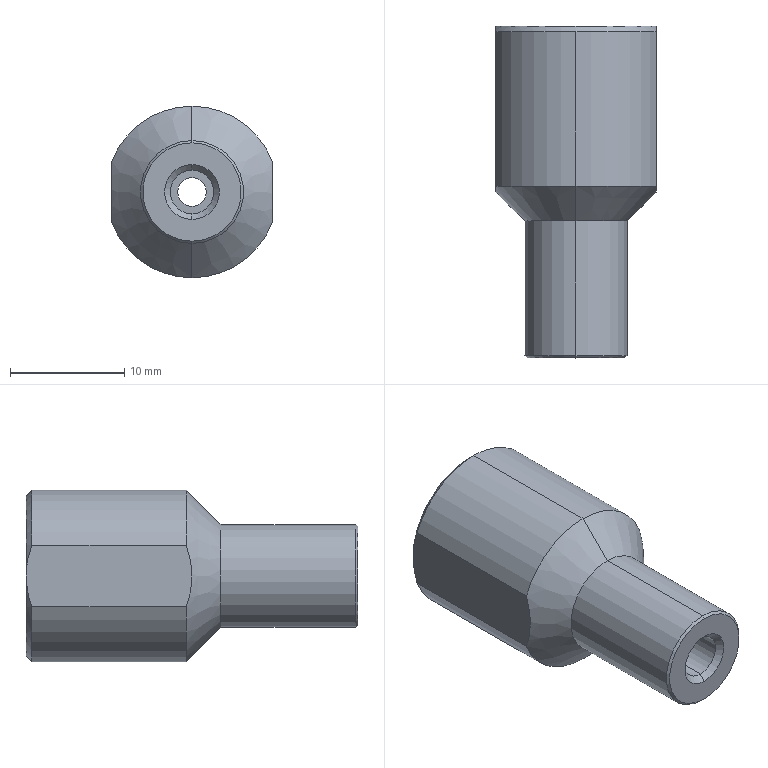Part | SolidWorks | features Chamfer 4, ICE 4, Extrusion 1, HoleWzd 1 | 1 solid | 27 faces | box 14 x 29 x 15 mm | volume 2672 mm3 | cylinder 11 | cone 11 | plane 5 | commonest cylinder face diameters 15 x3 2.5 x2 3.8 x2 8.5 x2 9 x2
STEP:
#1=CARTESIAN_POINT('',(0.,-12.,-4.25));
#2=VERTEX_POINT('',#1);
#3=CARTESIAN_POINT('',(0.,-12.,4.25));
#4=VERTEX_POINT('',#3);
#5=CARTESIAN_POINT('',(0.,-12.,0.));
#6=DIRECTION('',(0.,1.,0.));
#7=DIRECTION('',(0.,0.,1.));
#8=AXIS2_PLACEMENT_3D('',#5,#6,#7);
#9=CIRCLE('',#8,4.25);
#10=EDGE_CURVE('',#2,#4,#9,.T.);
#11=ORIENTED_EDGE('',*,*,#10,.F.);
#12=CARTESIAN_POINT('',(0.,0.,-4.25));
#13=VERTEX_POINT('',#12);
#14=CARTESIAN_POINT('',(0.,0.,-4.25));
#15=DIRECTION('',(0.,1.,0.));
#16=VECTOR('',#15,1000.);
#17=LINE('',#14,#16);
#18=EDGE_CURVE('',#2,#13,#17,.T.);
#19=ORIENTED_EDGE('',*,*,#18,.T.);
#20=CARTESIAN_POINT('',(0.,0.,4.25));
#21=VERTEX_POINT('',#20);
#22=CARTESIAN_POINT('',(0.,0.,0.));
#23=DIRECTION('',(0.,1.,0.));
#24=DIRECTION('',(0.,0.,1.));
#25=AXIS2_PLACEMENT_3D('',#22,#23,#24);
#26=CIRCLE('',#25,4.25);
#27=EDGE_CURVE('',#13,#21,#26,.T.);
#28=ORIENTED_EDGE('',*,*,#27,.T.);
#29=CARTESIAN_POINT('',(0.,0.,4.25));
#30=DIRECTION('',(0.,1.,0.));
#31=VECTOR('',#30,1000.);
#32=LINE('',#29,#31);
#33=EDGE_CURVE('',#4,#21,#32,.T.);
#34=ORIENTED_EDGE('',*,*,#33,.F.);
#35=EDGE_LOOP('',(#11,#19,#28,#34));
#36=FACE_OUTER_BOUND('',#35,.T.);
#37=CARTESIAN_POINT('',(0.,0.,0.));
#38=DIRECTION('',(0.,1.,0.));
#39=DIRECTION('',(0.,0.,1.));
#40=AXIS2_PLACEMENT_3D('',#37,#38,#39);
#41=CYLINDRICAL_SURFACE('',#40,4.25);
#42=ADVANCED_FACE('',(#36),#41,.F.);
#43=CARTESIAN_POINT('',(0.,-13.803,-1.25));
#44=VERTEX_POINT('',#43);
#45=CARTESIAN_POINT('',(0.,-13.803,1.25));
#46=VERTEX_POINT('',#45);
#47=CARTESIAN_POINT('',(0.,-13.803,0.));
#48=DIRECTION('',(0.,1.,0.));
#49=DIRECTION('',(0.,0.,1.));
#50=AXIS2_PLACEMENT_3D('',#47,#48,#49);
#51=CIRCLE('',#50,1.25);
#52=EDGE_CURVE('',#44,#46,#51,.T.);
#53=ORIENTED_EDGE('',*,*,#52,.F.);
#54=CARTESIAN_POINT('',(0.,-12.,-4.25));
#55=DIRECTION('',(0.,0.515,-0.8572));
#56=VECTOR('',#55,1000.);
#57=LINE('',#54,#56);
#58=EDGE_CURVE('',#44,#2,#57,.T.);
#59=ORIENTED_EDGE('',*,*,#58,.T.);
#60=ORIENTED_EDGE('',*,*,#10,.T.);
#61=CARTESIAN_POINT('',(0.,-12.,4.25));
#62=DIRECTION('',(0.,0.515,0.8572));
#63=VECTOR('',#62,1000.);
#64=LINE('',#61,#63);
#65=EDGE_CURVE('',#46,#4,#64,.T.);
#66=ORIENTED_EDGE('',*,*,#65,.F.);
#67=EDGE_LOOP('',(#53,#59,#60,#66));
#68=FACE_OUTER_BOUND('',#67,.T.);
#69=CARTESIAN_POINT('',(0.,-12.,0.));
#70=DIRECTION('',(0.,1.,0.));
#71=DIRECTION('',(0.,0.,1.));
#72=AXIS2_PLACEMENT_3D('',#69,#70,#71);
#73=CONICAL_SURFACE('',#72,4.25,1.03);
#74=ADVANCED_FACE('',(#68),#73,.F.);
#75=CARTESIAN_POINT('',(0.,-29.,-4.3));
#76=VERTEX_POINT('',#75);
#77=CARTESIAN_POINT('',(0.,-29.,4.3));
#78=VERTEX_POINT('',#77);
#79=CARTESIAN_POINT('',(0.,-29.,0.));
#80=DIRECTION('',(0.,-1.,0.));
#81=DIRECTION('',(0.,0.,-1.));
#82=AXIS2_PLACEMENT_3D('',#79,#80,#81);
#83=CIRCLE('',#82,4.3);
#84=EDGE_CURVE('',#76,#78,#83,.T.);
#85=ORIENTED_EDGE('',*,*,#84,.F.);
#86=CARTESIAN_POINT('',(0.,-28.8,-4.5));
#87=VERTEX_POINT('',#86);
#88=CARTESIAN_POINT('',(0.,-29.,-4.3));
#89=DIRECTION('',(0.,0.7071,-0.7071));
#90=VECTOR('',#89,1000.);
#91=LINE('',#88,#90);
#92=EDGE_CURVE('',#76,#87,#91,.T.);
#93=ORIENTED_EDGE('',*,*,#92,.T.);
#94=CARTESIAN_POINT('',(0.,-28.8,4.5));
#95=VERTEX_POINT('',#94);
#96=CARTESIAN_POINT('',(0.,-28.8,0.));
#97=DIRECTION('',(0.,1.,0.));
#98=DIRECTION('',(0.,0.,-1.));
#99=AXIS2_PLACEMENT_3D('',#96,#97,#98);
#100=CIRCLE('',#99,4.5);
#101=EDGE_CURVE('',#95,#87,#100,.T.);
#102=ORIENTED_EDGE('',*,*,#101,.F.);
#103=CARTESIAN_POINT('',(0.,-29.,4.3));
#104=DIRECTION('',(0.,0.7071,0.7071));
#105=VECTOR('',#104,1000.);
#106=LINE('',#103,#105);
#107=EDGE_CURVE('',#78,#95,#106,.T.);
#108=ORIENTED_EDGE('',*,*,#107,.F.);
#109=EDGE_LOOP('',(#85,#93,#102,#108));
#110=FACE_OUTER_BOUND('',#109,.T.);
#111=CARTESIAN_POINT('',(0.,-29.,0.));
#112=DIRECTION('',(0.,1.,0.));
#113=DIRECTION('',(0.,0.,1.));
#114=AXIS2_PLACEMENT_3D('',#111,#112,#113);
#115=CONICAL_SURFACE('',#114,4.3,0.7854);
#116=ADVANCED_FACE('',(#110),#115,.T.);
#117=CARTESIAN_POINT('',(0.,-28.5,1.9));
#118=VERTEX_POINT('',#117);
#119=CARTESIAN_POINT('',(0.,-28.5,-1.9));
#120=VERTEX_POINT('',#119);
#121=CARTESIAN_POINT('',(0.,-28.5,0.));
#122=DIRECTION('',(0.,-1.,0.));
#123=DIRECTION('',(0.,0.,-1.));
#124=AXIS2_PLACEMENT_3D('',#121,#122,#123);
#125=CIRCLE('',#124,1.9);
#126=EDGE_CURVE('',#118,#120,#125,.T.);
#127=ORIENTED_EDGE('',*,*,#126,.F.);
#128=CARTESIAN_POINT('',(0.,-29.,2.4));
#129=VERTEX_POINT('',#128);
#130=CARTESIAN_POINT('',(0.,-28.5,1.9));
#131=DIRECTION('',(0.,-0.7071,0.7071));
#132=VECTOR('',#131,1000.);
#133=LINE('',#130,#132);
#134=EDGE_CURVE('',#118,#129,#133,.T.);
#135=ORIENTED_EDGE('',*,*,#134,.T.);
#136=CARTESIAN_POINT('',(0.,-29.,-2.4));
#137=VERTEX_POINT('',#136);
#138=CARTESIAN_POINT('',(0.,-29.,0.));
#139=DIRECTION('',(0.,1.,0.));
#140=DIRECTION('',(0.,0.,-1.));
#141=AXIS2_PLACEMENT_3D('',#138,#139,#140);
#142=CIRCLE('',#141,2.4);
#143=EDGE_CURVE('',#137,#129,#142,.T.);
#144=ORIENTED_EDGE('',*,*,#143,.F.);
#145=CARTESIAN_POINT('',(0.,-28.5,-1.9));
#146=DIRECTION('',(0.,-0.7071,-0.7071));
#147=VECTOR('',#146,1000.);
#148=LINE('',#145,#147);
#149=EDGE_CURVE('',#120,#137,#148,.T.);
#150=ORIENTED_EDGE('',*,*,#149,.F.);
#151=EDGE_LOOP('',(#127,#135,#144,#150));
#152=FACE_OUTER_BOUND('',#151,.T.);
#153=CARTESIAN_POINT('',(0.,-28.5,0.));
#154=DIRECTION('',(0.,-1.,0.));
#155=DIRECTION('',(0.,0.,-1.));
#156=AXIS2_PLACEMENT_3D('',#153,#154,#155);
#157=CONICAL_SURFACE('',#156,1.9,0.7854);
#158=ADVANCED_FACE('',(#152),#157,.F.);
#159=ORIENTED_EDGE('',*,*,#52,.T.);
#160=CARTESIAN_POINT('',(0.,-21.,1.25));
#161=VERTEX_POINT('',#160);
#162=CARTESIAN_POINT('',(0.,0.,1.25));
#163=DIRECTION('',(0.,-1.,0.));
#164=VECTOR('',#163,1000.);
#165=LINE('',#162,#164);
#166=EDGE_CURVE('',#46,#161,#165,.T.);
#167=ORIENTED_EDGE('',*,*,#166,.T.);
#168=CARTESIAN_POINT('',(0.,-21.,-1.25));
#169=VERTEX_POINT('',#168);
#170=CARTESIAN_POINT('',(0.,-21.,0.));
#171=DIRECTION('',(0.,-1.,0.));
#172=DIRECTION('',(0.,0.,-1.));
#173=AXIS2_PLACEMENT_3D('',#170,#171,#172);
#174=CIRCLE('',#173,1.25);
#175=EDGE_CURVE('',#161,#169,#174,.T.);
#176=ORIENTED_EDGE('',*,*,#175,.T.);
#177=CARTESIAN_POINT('',(0.,0.,-1.25));
#178=DIRECTION('',(0.,-1.,0.));
#179=VECTOR('',#178,1000.);
#180=LINE('',#177,#179);
#181=EDGE_CURVE('',#44,#169,#180,.T.);
#182=ORIENTED_EDGE('',*,*,#181,.F.);
#183=EDGE_LOOP('',(#159,#167,#176,#182));
#184=FACE_OUTER_BOUND('',#183,.T.);
#185=CARTESIAN_POINT('',(0.,0.,0.));
#186=DIRECTION('',(0.,-1.,0.));
#187=DIRECTION('',(0.,0.,-1.));
#188=AXIS2_PLACEMENT_3D('',#185,#186,#187);
#189=CYLINDRICAL_SURFACE('',#188,1.25);
#190=ADVANCED_FACE('',(#184),#189,.F.);
#191=CARTESIAN_POINT('',(0.,-17.,-4.5));
#192=VERTEX_POINT('',#191);
#193=CARTESIAN_POINT('',(0.,-17.,4.5));
#194=VERTEX_POINT('',#193);
#195=CARTESIAN_POINT('',(0.,-17.,0.));
#196=DIRECTION('',(0.,-1.,0.));
#197=DIRECTION('',(0.,0.,1.));
#198=AXIS2_PLACEMENT_3D('',#195,#196,#197);
#199=CIRCLE('',#198,4.5);
#200=EDGE_CURVE('',#192,#194,#199,.T.);
#201=ORIENTED_EDGE('',*,*,#200,.F.);
#202=CARTESIAN_POINT('',(0.,-14.,-7.5));
#203=VERTEX_POINT('',#202);
#204=CARTESIAN_POINT('',(0.,-14.,-7.5));
#205=DIRECTION('',(0.,0.7071,-0.7071));
#206=VECTOR('',#205,1000.);
#207=LINE('',#204,#206);
#208=EDGE_CURVE('',#192,#203,#207,.T.);
#209=ORIENTED_EDGE('',*,*,#208,.T.);
#210=CARTESIAN_POINT('',(7.,-14.,-2.693));
#211=VERTEX_POINT('',#210);
#212=CARTESIAN_POINT('',(0.,-14.,0.));
#213=DIRECTION('',(0.,1.,0.));
#214=DIRECTION('',(0.,0.,1.));
#215=AXIS2_PLACEMENT_3D('',#212,#213,#214);
#216=CIRCLE('',#215,7.5);
#217=EDGE_CURVE('',#211,#203,#216,.T.);
#218=ORIENTED_EDGE('',*,*,#217,.F.);
#219=CARTESIAN_POINT('',(7.,-14.,2.693));
#220=VERTEX_POINT('',#219);
#221=CARTESIAN_POINT('',(7.,-14.,2.693));
#222=CARTESIAN_POINT('',(7.,-14.155,2.26));
#223=CARTESIAN_POINT('',(7.,-14.282,1.816));
#224=CARTESIAN_POINT('',(7.,-14.453,0.9207));
#225=CARTESIAN_POINT('',(7.,-14.5,0.4668));
#226=CARTESIAN_POINT('',(7.,-14.5,-0.2249));
#227=CARTESIAN_POINT('',(7.,-14.489,-0.4564));
#228=CARTESIAN_POINT('',(7.,-14.444,-0.9134));
#229=CARTESIAN_POINT('',(7.,-14.411,-1.14));
#230=CARTESIAN_POINT('',(7.,-14.325,-1.59));
#231=CARTESIAN_POINT('',(7.,-14.272,-1.813));
#232=CARTESIAN_POINT('',(7.,-14.148,-2.257));
#233=CARTESIAN_POINT('',(7.,-14.077,-2.477));
#234=CARTESIAN_POINT('',(7.,-14.,-2.693));
#235=B_SPLINE_CURVE_WITH_KNOTS('',3,(#221,#222,#223,#224,#225,#226,#227,#228,#229,#230,#231,#232,#233,#234),.UNSPECIFIED.,.F.,.F.,(4,2,2,2,2,2,4),(0.02883,0.03019,0.03156,0.03224,0.03292,0.0336,0.03428),.UNSPECIFIED.);
#236=EDGE_CURVE('',#220,#211,#235,.T.);
#237=ORIENTED_EDGE('',*,*,#236,.F.);
#238=CARTESIAN_POINT('',(0.,-14.,7.5));
#239=VERTEX_POINT('',#238);
#240=CARTESIAN_POINT('',(0.,-14.,0.));
#241=DIRECTION('',(0.,1.,0.));
#242=DIRECTION('',(0.,0.,1.));
#243=AXIS2_PLACEMENT_3D('',#240,#241,#242);
#244=CIRCLE('',#243,7.5);
#245=EDGE_CURVE('',#239,#220,#244,.T.);
#246=ORIENTED_EDGE('',*,*,#245,.F.);
#247=CARTESIAN_POINT('',(0.,-14.,7.5));
#248=DIRECTION('',(0.,0.7071,0.7071));
#249=VECTOR('',#248,1000.);
#250=LINE('',#247,#249);
#251=EDGE_CURVE('',#194,#239,#250,.T.);
#252=ORIENTED_EDGE('',*,*,#251,.F.);
#253=EDGE_LOOP('',(#201,#209,#218,#237,#246,#252));
#254=FACE_OUTER_BOUND('',#253,.T.);
#255=CARTESIAN_POINT('',(0.,-14.,0.));
#256=DIRECTION('',(0.,1.,0.));
#257=DIRECTION('',(0.,0.,1.));
#258=AXIS2_PLACEMENT_3D('',#255,#256,#257);
#259=CONICAL_SURFACE('',#258,7.5,0.7854);
#260=ADVANCED_FACE('',(#254),#259,.T.);
#261=CARTESIAN_POINT('',(0.,-21.,1.9));
#262=VERTEX_POINT('',#261);
#263=CARTESIAN_POINT('',(0.,-21.,-1.9));
#264=VERTEX_POINT('',#263);
#265=CARTESIAN_POINT('',(0.,-21.,0.));
#266=DIRECTION('',(0.,-1.,0.));
#267=DIRECTION('',(0.,0.,-1.));
#268=AXIS2_PLACEMENT_3D('',#265,#266,#267);
#269=CIRCLE('',#268,1.9);
#270=EDGE_CURVE('',#262,#264,#269,.T.);
#271=ORIENTED_EDGE('',*,*,#270,.F.);
#272=CARTESIAN_POINT('',(0.,-21.,1.9));
#273=DIRECTION('',(0.,-1.,0.));
#274=VECTOR('',#273,1000.);
#275=LINE('',#272,#274);
#276=EDGE_CURVE('',#262,#118,#275,.T.);
#277=ORIENTED_EDGE('',*,*,#276,.T.);
#278=ORIENTED_EDGE('',*,*,#126,.T.);
#279=CARTESIAN_POINT('',(0.,-21.,-1.9));
#280=DIRECTION('',(0.,-1.,0.));
#281=VECTOR('',#280,1000.);
#282=LINE('',#279,#281);
#283=EDGE_CURVE('',#264,#120,#282,.T.);
#284=ORIENTED_EDGE('',*,*,#283,.F.);
#285=EDGE_LOOP('',(#271,#277,#278,#284));
#286=FACE_OUTER_BOUND('',#285,.T.);
#287=CARTESIAN_POINT('',(0.,-21.,0.));
#288=DIRECTION('',(0.,-1.,0.));
#289=DIRECTION('',(0.,0.,-1.));
#290=AXIS2_PLACEMENT_3D('',#287,#288,#289);
#291=CYLINDRICAL_SURFACE('',#290,1.9);
#292=ADVANCED_FACE('',(#286),#291,.F.);
#293=ORIENTED_EDGE('',*,*,#101,.T.);
#294=CARTESIAN_POINT('',(0.,-29.,-4.5));
#295=DIRECTION('',(0.,1.,0.));
#296=VECTOR('',#295,1000.);
#297=LINE('',#294,#296);
#298=EDGE_CURVE('',#87,#192,#297,.T.);
#299=ORIENTED_EDGE('',*,*,#298,.T.);
#300=ORIENTED_EDGE('',*,*,#200,.T.);
#301=CARTESIAN_POINT('',(0.,-29.,4.5));
#302=DIRECTION('',(0.,1.,0.));
#303=VECTOR('',#302,1000.);
#304=LINE('',#301,#303);
#305=EDGE_CURVE('',#95,#194,#304,.T.);
#306=ORIENTED_EDGE('',*,*,#305,.F.);
#307=EDGE_LOOP('',(#293,#299,#300,#306));
#308=FACE_OUTER_BOUND('',#307,.T.);
#309=CARTESIAN_POINT('',(0.,-29.,0.));
#310=DIRECTION('',(0.,1.,0.));
#311=DIRECTION('',(0.,0.,1.));
#312=AXIS2_PLACEMENT_3D('',#309,#310,#311);
#313=CYLINDRICAL_SURFACE('',#312,4.5);
#314=ADVANCED_FACE('',(#308),#313,.T.);
#315=CARTESIAN_POINT('',(0.,0.,-7.));
#316=VERTEX_POINT('',#315);
#317=CARTESIAN_POINT('',(-7.,0.,0.));
#318=VERTEX_POINT('',#317);
#319=CARTESIAN_POINT('',(0.,0.,0.));
#320=DIRECTION('',(0.,1.,0.));
#321=DIRECTION('',(0.,0.,1.));
#322=AXIS2_PLACEMENT_3D('',#319,#320,#321);
#323=CIRCLE('',#322,7.);
#324=EDGE_CURVE('',#316,#318,#323,.T.);
#325=ORIENTED_EDGE('',*,*,#324,.F.);
#326=CARTESIAN_POINT('',(0.,-0.5,-7.5));
#327=VERTEX_POINT('',#326);
#328=CARTESIAN_POINT('',(0.,0.,-7.));
#329=DIRECTION('',(0.,-0.7071,-0.7071));
#330=VECTOR('',#329,1000.);
#331=LINE('',#328,#330);
#332=EDGE_CURVE('',#316,#327,#331,.T.);
#333=ORIENTED_EDGE('',*,*,#332,.T.);
#334=CARTESIAN_POINT('',(-7.,-0.5,-2.693));
#335=VERTEX_POINT('',#334);
#336=CARTESIAN_POINT('',(0.,-0.5,0.));
#337=DIRECTION('',(0.,-1.,0.));
#338=DIRECTION('',(0.,0.,1.));
#339=AXIS2_PLACEMENT_3D('',#336,#337,#338);
#340=CIRCLE('',#339,7.5);
#341=EDGE_CURVE('',#335,#327,#340,.T.);
#342=ORIENTED_EDGE('',*,*,#341,.F.);
#343=CARTESIAN_POINT('',(-7.,0.,0.));
#344=CARTESIAN_POINT('',(-7.,0.,-0.4603));
#345=CARTESIAN_POINT('',(-7.,-0.04574,-0.9154));
#346=CARTESIAN_POINT('',(-7.,-0.2183,-1.816));
#347=CARTESIAN_POINT('',(-7.,-0.3456,-2.263));
#348=CARTESIAN_POINT('',(-7.,-0.5,-2.693));
#349=B_SPLINE_CURVE_WITH_KNOTS('',3,(#343,#344,#345,#346,#347,#348),.UNSPECIFIED.,.F.,.F.,(4,2,4),(0.008783,0.01014,0.0115),.UNSPECIFIED.);
#350=EDGE_CURVE('',#318,#335,#349,.T.);
#351=ORIENTED_EDGE('',*,*,#350,.F.);
#352=EDGE_LOOP('',(#325,#333,#342,#351));
#353=FACE_OUTER_BOUND('',#352,.T.);
#354=CARTESIAN_POINT('',(0.,0.,0.));
#355=DIRECTION('',(0.,-1.,0.));
#356=DIRECTION('',(0.,0.,-1.));
#357=AXIS2_PLACEMENT_3D('',#354,#355,#356);
#358=CONICAL_SURFACE('',#357,7.,0.7854);
#359=ADVANCED_FACE('',(#353),#358,.T.);
#360=CARTESIAN_POINT('',(-7.,-14.,2.693));
#361=VERTEX_POINT('',#360);
#362=CARTESIAN_POINT('',(0.,-14.,0.));
#363=DIRECTION('',(0.,1.,0.));
#364=DIRECTION('',(0.,0.,1.));
#365=AXIS2_PLACEMENT_3D('',#362,#363,#364);
#366=CIRCLE('',#365,7.5);
#367=EDGE_CURVE('',#361,#239,#366,.T.);
#368=ORIENTED_EDGE('',*,*,#367,.T.);
#369=CARTESIAN_POINT('',(0.,-0.5,7.5));
#370=VERTEX_POINT('',#369);
#371=CARTESIAN_POINT('',(0.,-17.,7.5));
#372=DIRECTION('',(0.,1.,0.));
#373=VECTOR('',#372,1000.);
#374=LINE('',#371,#373);
#375=EDGE_CURVE('',#239,#370,#374,.T.);
#376=ORIENTED_EDGE('',*,*,#375,.T.);
#377=CARTESIAN_POINT('',(-7.,-0.5,2.693));
#378=VERTEX_POINT('',#377);
#379=CARTESIAN_POINT('',(0.,-0.5,0.));
#380=DIRECTION('',(0.,-1.,0.));
#381=DIRECTION('',(0.,0.,1.));
#382=AXIS2_PLACEMENT_3D('',#379,#380,#381);
#383=CIRCLE('',#382,7.5);
#384=EDGE_CURVE('',#370,#378,#383,.T.);
#385=ORIENTED_EDGE('',*,*,#384,.T.);
#386=CARTESIAN_POINT('',(-7.,-17.,2.693));
#387=DIRECTION('',(0.,1.,0.));
#388=VECTOR('',#387,1000.);
#389=LINE('',#386,#388);
#390=EDGE_CURVE('',#361,#378,#389,.T.);
#391=ORIENTED_EDGE('',*,*,#390,.F.);
#392=EDGE_LOOP('',(#368,#376,#385,#391));
#393=FACE_OUTER_BOUND('',#392,.T.);
#394=CARTESIAN_POINT('',(0.,-17.,0.));
#395=DIRECTION('',(0.,1.,0.));
#396=DIRECTION('',(0.,0.,1.));
#397=AXIS2_PLACEMENT_3D('',#394,#395,#396);
#398=CYLINDRICAL_SURFACE('',#397,7.5);
#399=ADVANCED_FACE('',(#393),#398,.T.);
#400=ORIENTED_EDGE('',*,*,#375,.F.);
#401=ORIENTED_EDGE('',*,*,#245,.T.);
#402=CARTESIAN_POINT('',(7.,-0.5,2.693));
#403=VERTEX_POINT('',#402);
#404=CARTESIAN_POINT('',(7.,-17.,2.693));
#405=DIRECTION('',(0.,-1.,0.));
#406=VECTOR('',#405,1000.);
#407=LINE('',#404,#406);
#408=EDGE_CURVE('',#403,#220,#407,.T.);
#409=ORIENTED_EDGE('',*,*,#408,.F.);
#410=CARTESIAN_POINT('',(0.,-0.5,0.));
#411=DIRECTION('',(0.,-1.,0.));
#412=DIRECTION('',(0.,0.,1.));
#413=AXIS2_PLACEMENT_3D('',#410,#411,#412);
#414=CIRCLE('',#413,7.5);
#415=EDGE_CURVE('',#403,#370,#414,.T.);
#416=ORIENTED_EDGE('',*,*,#415,.T.);
#417=EDGE_LOOP('',(#400,#401,#409,#416));
#418=FACE_OUTER_BOUND('',#417,.T.);
#419=CARTESIAN_POINT('',(0.,-17.,0.));
#420=DIRECTION('',(0.,1.,0.));
#421=DIRECTION('',(0.,0.,1.));
#422=AXIS2_PLACEMENT_3D('',#419,#420,#421);
#423=CYLINDRICAL_SURFACE('',#422,7.5);
#424=ADVANCED_FACE('',(#418),#423,.T.);
#425=ORIENTED_EDGE('',*,*,#332,.F.);
#426=CARTESIAN_POINT('',(7.,0.,0.));
#427=VERTEX_POINT('',#426);
#428=CARTESIAN_POINT('',(0.,0.,0.));
#429=DIRECTION('',(0.,1.,0.));
#430=DIRECTION('',(0.,0.,1.));
#431=AXIS2_PLACEMENT_3D('',#428,#429,#430);
#432=CIRCLE('',#431,7.);
#433=EDGE_CURVE('',#427,#316,#432,.T.);
#434=ORIENTED_EDGE('',*,*,#433,.F.);
#435=CARTESIAN_POINT('',(7.,-0.5,-2.693));
#436=VERTEX_POINT('',#435);
#437=CARTESIAN_POINT('',(7.,-0.5,-2.693));
#438=CARTESIAN_POINT('',(7.,-0.3456,-2.263));
#439=CARTESIAN_POINT('',(7.,-0.2183,-1.816));
#440=CARTESIAN_POINT('',(7.,-0.04574,-0.9154));
#441=CARTESIAN_POINT('',(7.,0.,-0.4603));
#442=CARTESIAN_POINT('',(7.,0.,0.));
#443=B_SPLINE_CURVE_WITH_KNOTS('',3,(#437,#438,#439,#440,#441,#442),.UNSPECIFIED.,.F.,.F.,(4,2,4),(0.002778,0.004145,0.005512),.UNSPECIFIED.);
#444=EDGE_CURVE('',#436,#427,#443,.T.);
#445=ORIENTED_EDGE('',*,*,#444,.F.);
#446=CARTESIAN_POINT('',(0.,-0.5,0.));
#447=DIRECTION('',(0.,-1.,0.));
#448=DIRECTION('',(0.,0.,1.));
#449=AXIS2_PLACEMENT_3D('',#446,#447,#448);
#450=CIRCLE('',#449,7.5);
#451=EDGE_CURVE('',#327,#436,#450,.T.);
#452=ORIENTED_EDGE('',*,*,#451,.F.);
#453=EDGE_LOOP('',(#425,#434,#445,#452));
#454=FACE_OUTER_BOUND('',#453,.T.);
#455=CARTESIAN_POINT('',(0.,0.,0.));
#456=DIRECTION('',(0.,-1.,0.));
#457=DIRECTION('',(0.,0.,-1.));
#458=AXIS2_PLACEMENT_3D('',#455,#456,#457);
#459=CONICAL_SURFACE('',#458,7.,0.7854);
#460=ADVANCED_FACE('',(#454),#459,.T.);
#461=CARTESIAN_POINT('',(7.,-17.,-2.693));
#462=DIRECTION('',(0.,1.,0.));
#463=VECTOR('',#462,1000.);
#464=LINE('',#461,#463);
#465=EDGE_CURVE('',#211,#436,#464,.T.);
#466=ORIENTED_EDGE('',*,*,#465,.F.);
#467=ORIENTED_EDGE('',*,*,#217,.T.);
#468=CARTESIAN_POINT('',(-7.,-14.,-2.693));
#469=VERTEX_POINT('',#468);
#470=CARTESIAN_POINT('',(0.,-14.,0.));
#471=DIRECTION('',(0.,1.,0.));
#472=DIRECTION('',(0.,0.,1.));
#473=AXIS2_PLACEMENT_3D('',#470,#471,#472);
#474=CIRCLE('',#473,7.5);
#475=EDGE_CURVE('',#203,#469,#474,.T.);
#476=ORIENTED_EDGE('',*,*,#475,.T.);
#477=CARTESIAN_POINT('',(-7.,-17.,-2.693));
#478=DIRECTION('',(0.,-1.,0.));
#479=VECTOR('',#478,1000.);
#480=LINE('',#477,#479);
#481=EDGE_CURVE('',#335,#469,#480,.T.);
#482=ORIENTED_EDGE('',*,*,#481,.F.);
#483=ORIENTED_EDGE('',*,*,#341,.T.);
#484=ORIENTED_EDGE('',*,*,#451,.T.);
#485=EDGE_LOOP('',(#466,#467,#476,#482,#483,#484));
#486=FACE_OUTER_BOUND('',#485,.T.);
#487=CARTESIAN_POINT('',(0.,-17.,0.));
#488=DIRECTION('',(0.,1.,0.));
#489=DIRECTION('',(0.,0.,1.));
#490=AXIS2_PLACEMENT_3D('',#487,#488,#489);
#491=CYLINDRICAL_SURFACE('',#490,7.5);
#492=ADVANCED_FACE('',(#486),#491,.T.);
#493=CARTESIAN_POINT('',(0.,0.,0.));
#494=DIRECTION('',(0.,1.,0.));
#495=DIRECTION('',(0.,0.,1.));
#496=AXIS2_PLACEMENT_3D('',#493,#494,#495);
#497=CIRCLE('',#496,4.25);
#498=EDGE_CURVE('',#21,#13,#497,.T.);
#499=ORIENTED_EDGE('',*,*,#498,.F.);
#500=ORIENTED_EDGE('',*,*,#27,.F.);
#501=EDGE_LOOP('',(#499,#500));
#502=FACE_BOUND('',#501,.T.);
#503=CARTESIAN_POINT('',(0.,0.,0.));
#504=DIRECTION('',(0.,1.,0.));
#505=DIRECTION('',(0.,0.,1.));
#506=AXIS2_PLACEMENT_3D('',#503,#504,#505);
#507=CIRCLE('',#506,7.);
#508=EDGE_CURVE('',#318,#427,#507,.T.);
#509=ORIENTED_EDGE('',*,*,#508,.T.);
#510=ORIENTED_EDGE('',*,*,#433,.T.);
#511=ORIENTED_EDGE('',*,*,#324,.T.);
#512=EDGE_LOOP('',(#509,#510,#511));
#513=FACE_OUTER_BOUND('',#512,.T.);
#514=CARTESIAN_POINT('',(0.,0.,0.));
#515=DIRECTION('',(0.,1.,0.));
#516=DIRECTION('',(0.,0.,1.));
#517=AXIS2_PLACEMENT_3D('',#514,#515,#516);
#518=PLANE('',#517);
#519=ADVANCED_FACE('',(#502,#513),#518,.T.);
#520=ORIENTED_EDGE('',*,*,#298,.F.);
#521=CARTESIAN_POINT('',(0.,-28.8,0.));
#522=DIRECTION('',(0.,1.,0.));
#523=DIRECTION('',(0.,0.,-1.));
#524=AXIS2_PLACEMENT_3D('',#521,#522,#523);
#525=CIRCLE('',#524,4.5);
#526=EDGE_CURVE('',#87,#95,#525,.T.);
#527=ORIENTED_EDGE('',*,*,#526,.T.);
#528=ORIENTED_EDGE('',*,*,#305,.T.);
#529=CARTESIAN_POINT('',(0.,-17.,0.));
#530=DIRECTION('',(0.,-1.,0.));
#531=DIRECTION('',(0.,0.,1.));
#532=AXIS2_PLACEMENT_3D('',#529,#530,#531);
#533=CIRCLE('',#532,4.5);
#534=EDGE_CURVE('',#194,#192,#533,.T.);
#535=ORIENTED_EDGE('',*,*,#534,.T.);
#536=EDGE_LOOP('',(#520,#527,#528,#535));
#537=FACE_OUTER_BOUND('',#536,.T.);
#538=CARTESIAN_POINT('',(0.,-29.,0.));
#539=DIRECTION('',(0.,1.,0.));
#540=DIRECTION('',(0.,0.,1.));
#541=AXIS2_PLACEMENT_3D('',#538,#539,#540);
#542=CYLINDRICAL_SURFACE('',#541,4.5);
#543=ADVANCED_FACE('',(#537),#542,.T.);
#544=CARTESIAN_POINT('',(0.,-29.,0.));
#545=DIRECTION('',(0.,-1.,0.));
#546=DIRECTION('',(0.,0.,-1.));
#547=AXIS2_PLACEMENT_3D('',#544,#545,#546);
#548=CIRCLE('',#547,4.3);
#549=EDGE_CURVE('',#78,#76,#548,.T.);
#550=ORIENTED_EDGE('',*,*,#549,.T.);
#551=ORIENTED_EDGE('',*,*,#84,.T.);
#552=EDGE_LOOP('',(#550,#551));
#553=FACE_OUTER_BOUND('',#552,.T.);
#554=ORIENTED_EDGE('',*,*,#143,.T.);
#555=CARTESIAN_POINT('',(0.,-29.,0.));
#556=DIRECTION('',(0.,1.,0.));
#557=DIRECTION('',(0.,0.,-1.));
#558=AXIS2_PLACEMENT_3D('',#555,#556,#557);
#559=CIRCLE('',#558,2.4);
#560=EDGE_CURVE('',#129,#137,#559,.T.);
#561=ORIENTED_EDGE('',*,*,#560,.T.);
#562=EDGE_LOOP('',(#554,#561));
#563=FACE_BOUND('',#562,.T.);
#564=CARTESIAN_POINT('',(0.,-29.,0.));
#565=DIRECTION('',(0.,-1.,0.));
#566=DIRECTION('',(0.,0.,-1.));
#567=AXIS2_PLACEMENT_3D('',#564,#565,#566);
#568=PLANE('',#567);
#569=ADVANCED_FACE('',(#553,#563),#568,.T.);
#570=ORIENTED_EDGE('',*,*,#276,.F.);
#571=CARTESIAN_POINT('',(0.,-21.,0.));
#572=DIRECTION('',(0.,-1.,0.));
#573=DIRECTION('',(0.,0.,-1.));
#574=AXIS2_PLACEMENT_3D('',#571,#572,#573);
#575=CIRCLE('',#574,1.9);
#576=EDGE_CURVE('',#264,#262,#575,.T.);
#577=ORIENTED_EDGE('',*,*,#576,.F.);
#578=ORIENTED_EDGE('',*,*,#283,.T.);
#579=CARTESIAN_POINT('',(0.,-28.5,0.));
#580=DIRECTION('',(0.,-1.,0.));
#581=DIRECTION('',(0.,0.,-1.));
#582=AXIS2_PLACEMENT_3D('',#579,#580,#581);
#583=CIRCLE('',#582,1.9);
#584=EDGE_CURVE('',#120,#118,#583,.T.);
#585=ORIENTED_EDGE('',*,*,#584,.T.);
#586=EDGE_LOOP('',(#570,#577,#578,#585));
#587=FACE_OUTER_BOUND('',#586,.T.);
#588=CARTESIAN_POINT('',(0.,-21.,0.));
#589=DIRECTION('',(0.,-1.,0.));
#590=DIRECTION('',(0.,0.,-1.));
#591=AXIS2_PLACEMENT_3D('',#588,#589,#590);
#592=CYLINDRICAL_SURFACE('',#591,1.9);
#593=ADVANCED_FACE('',(#587),#592,.F.);
#594=CARTESIAN_POINT('',(0.,-21.,0.));
#595=DIRECTION('',(0.,-1.,0.));
#596=DIRECTION('',(0.,0.,-1.));
#597=AXIS2_PLACEMENT_3D('',#594,#595,#596);
#598=CIRCLE('',#597,1.25);
#599=EDGE_CURVE('',#169,#161,#598,.T.);
#600=ORIENTED_EDGE('',*,*,#599,.F.);
#601=ORIENTED_EDGE('',*,*,#175,.F.);
#602=EDGE_LOOP('',(#600,#601));
#603=FACE_BOUND('',#602,.T.);
#604=ORIENTED_EDGE('',*,*,#576,.T.);
#605=ORIENTED_EDGE('',*,*,#270,.T.);
#606=EDGE_LOOP('',(#604,#605));
#607=FACE_OUTER_BOUND('',#606,.T.);
#608=CARTESIAN_POINT('',(0.,-21.,0.));
#609=DIRECTION('',(0.,-1.,0.));
#610=DIRECTION('',(0.,0.,-1.));
#611=AXIS2_PLACEMENT_3D('',#608,#609,#610);
#612=PLANE('',#611);
#613=ADVANCED_FACE('',(#603,#607),#612,.T.);
#614=ORIENTED_EDGE('',*,*,#208,.F.);
#615=ORIENTED_EDGE('',*,*,#534,.F.);
#616=ORIENTED_EDGE('',*,*,#251,.T.);
#617=ORIENTED_EDGE('',*,*,#367,.F.);
#618=CARTESIAN_POINT('',(-7.,-14.,-2.693));
#619=CARTESIAN_POINT('',(-7.,-14.077,-2.477));
#620=CARTESIAN_POINT('',(-7.,-14.148,-2.257));
#621=CARTESIAN_POINT('',(-7.,-14.272,-1.813));
#622=CARTESIAN_POINT('',(-7.,-14.325,-1.59));
#623=CARTESIAN_POINT('',(-7.,-14.411,-1.14));
#624=CARTESIAN_POINT('',(-7.,-14.444,-0.9134));
#625=CARTESIAN_POINT('',(-7.,-14.489,-0.4564));
#626=CARTESIAN_POINT('',(-7.,-14.5,-0.2249));
#627=CARTESIAN_POINT('',(-7.,-14.5,0.4668));
#628=CARTESIAN_POINT('',(-7.,-14.453,0.9207));
#629=CARTESIAN_POINT('',(-7.,-14.282,1.816));
#630=CARTESIAN_POINT('',(-7.,-14.155,2.26));
#631=CARTESIAN_POINT('',(-7.,-14.,2.693));
#632=B_SPLINE_CURVE_WITH_KNOTS('',3,(#618,#619,#620,#621,#622,#623,#624,#625,#626,#627,#628,#629,#630,#631),.UNSPECIFIED.,.F.,.F.,(4,2,2,2,2,2,4),(0.02669,0.02737,0.02805,0.02873,0.02941,0.03076,0.03212),.UNSPECIFIED.);
#633=EDGE_CURVE('',#469,#361,#632,.T.);
#634=ORIENTED_EDGE('',*,*,#633,.F.);
#635=ORIENTED_EDGE('',*,*,#475,.F.);
#636=EDGE_LOOP('',(#614,#615,#616,#617,#634,#635));
#637=FACE_OUTER_BOUND('',#636,.T.);
#638=CARTESIAN_POINT('',(0.,-14.,0.));
#639=DIRECTION('',(0.,1.,0.));
#640=DIRECTION('',(0.,0.,1.));
#641=AXIS2_PLACEMENT_3D('',#638,#639,#640);
#642=CONICAL_SURFACE('',#641,7.5,0.7854);
#643=ADVANCED_FACE('',(#637),#642,.T.);
#644=ORIENTED_EDGE('',*,*,#166,.F.);
#645=CARTESIAN_POINT('',(0.,-13.803,0.));
#646=DIRECTION('',(0.,1.,0.));
#647=DIRECTION('',(0.,0.,1.));
#648=AXIS2_PLACEMENT_3D('',#645,#646,#647);
#649=CIRCLE('',#648,1.25);
#650=EDGE_CURVE('',#46,#44,#649,.T.);
#651=ORIENTED_EDGE('',*,*,#650,.T.);
#652=ORIENTED_EDGE('',*,*,#181,.T.);
#653=ORIENTED_EDGE('',*,*,#599,.T.);
#654=EDGE_LOOP('',(#644,#651,#652,#653));
#655=FACE_OUTER_BOUND('',#654,.T.);
#656=CARTESIAN_POINT('',(0.,0.,0.));
#657=DIRECTION('',(0.,-1.,0.));
#658=DIRECTION('',(0.,0.,-1.));
#659=AXIS2_PLACEMENT_3D('',#656,#657,#658);
#660=CYLINDRICAL_SURFACE('',#659,1.25);
#661=ADVANCED_FACE('',(#655),#660,.F.);
#662=CARTESIAN_POINT('',(7.,0.,0.));
#663=CARTESIAN_POINT('',(7.,0.,0.2303));
#664=CARTESIAN_POINT('',(7.,-0.01156,0.4621));
#665=CARTESIAN_POINT('',(7.,-0.05641,0.919));
#666=CARTESIAN_POINT('',(7.,-0.08965,1.145));
#667=CARTESIAN_POINT('',(7.,-0.2188,1.818));
#668=CARTESIAN_POINT('',(7.,-0.3441,2.258));
#669=CARTESIAN_POINT('',(7.,-0.5,2.693));
#670=B_SPLINE_CURVE_WITH_KNOTS('',3,(#662,#663,#664,#665,#666,#667,#668,#669),.UNSPECIFIED.,.F.,.F.,(4,2,2,4),(0.005512,0.006196,0.00688,0.008248),.UNSPECIFIED.);
#671=EDGE_CURVE('',#427,#403,#670,.T.);
#672=ORIENTED_EDGE('',*,*,#671,.F.);
#673=ORIENTED_EDGE('',*,*,#508,.F.);
#674=CARTESIAN_POINT('',(-7.,-0.5,2.693));
#675=CARTESIAN_POINT('',(-7.,-0.3441,2.258));
#676=CARTESIAN_POINT('',(-7.,-0.2188,1.818));
#677=CARTESIAN_POINT('',(-7.,-0.08965,1.145));
#678=CARTESIAN_POINT('',(-7.,-0.05641,0.919));
#679=CARTESIAN_POINT('',(-7.,-0.01156,0.4621));
#680=CARTESIAN_POINT('',(-7.,0.,0.2303));
#681=CARTESIAN_POINT('',(-7.,0.,0.));
#682=B_SPLINE_CURVE_WITH_KNOTS('',3,(#674,#675,#676,#677,#678,#679,#680,#681),.UNSPECIFIED.,.F.,.F.,(4,2,2,4),(0.006062,0.007422,0.008103,0.008783),.UNSPECIFIED.);
#683=EDGE_CURVE('',#378,#318,#682,.T.);
#684=ORIENTED_EDGE('',*,*,#683,.F.);
#685=ORIENTED_EDGE('',*,*,#384,.F.);
#686=ORIENTED_EDGE('',*,*,#415,.F.);
#687=EDGE_LOOP('',(#672,#673,#684,#685,#686));
#688=FACE_OUTER_BOUND('',#687,.T.);
#689=CARTESIAN_POINT('',(0.,0.,0.));
#690=DIRECTION('',(0.,-1.,0.));
#691=DIRECTION('',(0.,0.,-1.));
#692=AXIS2_PLACEMENT_3D('',#689,#690,#691);
#693=CONICAL_SURFACE('',#692,7.,0.7854);
#694=ADVANCED_FACE('',(#688),#693,.T.);
#695=ORIENTED_EDGE('',*,*,#633,.T.);
#696=ORIENTED_EDGE('',*,*,#390,.T.);
#697=ORIENTED_EDGE('',*,*,#683,.T.);
#698=ORIENTED_EDGE('',*,*,#350,.T.);
#699=ORIENTED_EDGE('',*,*,#481,.T.);
#700=EDGE_LOOP('',(#695,#696,#697,#698,#699));
#701=FACE_OUTER_BOUND('',#700,.T.);
#702=CARTESIAN_POINT('',(-7.,27.72,-7.5));
#703=DIRECTION('',(1.,0.,0.));
#704=DIRECTION('',(0.,1.,0.));
#705=AXIS2_PLACEMENT_3D('',#702,#703,#704);
#706=PLANE('',#705);
#707=ADVANCED_FACE('',(#701),#706,.F.);
#708=ORIENTED_EDGE('',*,*,#236,.T.);
#709=ORIENTED_EDGE('',*,*,#465,.T.);
#710=ORIENTED_EDGE('',*,*,#444,.T.);
#711=ORIENTED_EDGE('',*,*,#671,.T.);
#712=ORIENTED_EDGE('',*,*,#408,.T.);
#713=EDGE_LOOP('',(#708,#709,#710,#711,#712));
#714=FACE_OUTER_BOUND('',#713,.T.);
#715=CARTESIAN_POINT('',(7.,34.298,-7.5));
#716=DIRECTION('',(-1.,0.,0.));
#717=DIRECTION('',(0.,-1.,0.));
#718=AXIS2_PLACEMENT_3D('',#715,#716,#717);
#719=PLANE('',#718);
#720=ADVANCED_FACE('',(#714),#719,.F.);
#721=ORIENTED_EDGE('',*,*,#134,.F.);
#722=ORIENTED_EDGE('',*,*,#584,.F.);
#723=ORIENTED_EDGE('',*,*,#149,.T.);
#724=ORIENTED_EDGE('',*,*,#560,.F.);
#725=EDGE_LOOP('',(#721,#722,#723,#724));
#726=FACE_OUTER_BOUND('',#725,.T.);
#727=CARTESIAN_POINT('',(0.,-28.5,0.));
#728=DIRECTION('',(0.,-1.,0.));
#729=DIRECTION('',(0.,0.,-1.));
#730=AXIS2_PLACEMENT_3D('',#727,#728,#729);
#731=CONICAL_SURFACE('',#730,1.9,0.7854);
#732=ADVANCED_FACE('',(#726),#731,.F.);
#733=ORIENTED_EDGE('',*,*,#92,.F.);
#734=ORIENTED_EDGE('',*,*,#549,.F.);
#735=ORIENTED_EDGE('',*,*,#107,.T.);
#736=ORIENTED_EDGE('',*,*,#526,.F.);
#737=EDGE_LOOP('',(#733,#734,#735,#736));
#738=FACE_OUTER_BOUND('',#737,.T.);
#739=CARTESIAN_POINT('',(0.,-29.,0.));
#740=DIRECTION('',(0.,1.,0.));
#741=DIRECTION('',(0.,0.,1.));
#742=AXIS2_PLACEMENT_3D('',#739,#740,#741);
#743=CONICAL_SURFACE('',#742,4.3,0.7854);
#744=ADVANCED_FACE('',(#738),#743,.T.);
#745=ORIENTED_EDGE('',*,*,#58,.F.);
#746=ORIENTED_EDGE('',*,*,#650,.F.);
#747=ORIENTED_EDGE('',*,*,#65,.T.);
#748=CARTESIAN_POINT('',(0.,-12.,0.));
#749=DIRECTION('',(0.,1.,0.));
#750=DIRECTION('',(0.,0.,1.));
#751=AXIS2_PLACEMENT_3D('',#748,#749,#750);
#752=CIRCLE('',#751,4.25);
#753=EDGE_CURVE('',#4,#2,#752,.T.);
#754=ORIENTED_EDGE('',*,*,#753,.T.);
#755=EDGE_LOOP('',(#745,#746,#747,#754));
#756=FACE_OUTER_BOUND('',#755,.T.);
#757=CARTESIAN_POINT('',(0.,-12.,0.));
#758=DIRECTION('',(0.,1.,0.));
#759=DIRECTION('',(0.,0.,1.));
#760=AXIS2_PLACEMENT_3D('',#757,#758,#759);
#761=CONICAL_SURFACE('',#760,4.25,1.03);
#762=ADVANCED_FACE('',(#756),#761,.F.);
#763=ORIENTED_EDGE('',*,*,#18,.F.);
#764=ORIENTED_EDGE('',*,*,#753,.F.);
#765=ORIENTED_EDGE('',*,*,#33,.T.);
#766=ORIENTED_EDGE('',*,*,#498,.T.);
#767=EDGE_LOOP('',(#763,#764,#765,#766));
#768=FACE_OUTER_BOUND('',#767,.T.);
#769=CARTESIAN_POINT('',(0.,0.,0.));
#770=DIRECTION('',(0.,1.,0.));
#771=DIRECTION('',(0.,0.,1.));
#772=AXIS2_PLACEMENT_3D('',#769,#770,#771);
#773=CYLINDRICAL_SURFACE('',#772,4.25);
#774=ADVANCED_FACE('',(#768),#773,.F.);
#775=CLOSED_SHELL('',(#42,#74,#116,#158,#190,#260,#292,#314,#359,#399,#424,#460,#492,#519,#543,#569,#593,#613,#643,#661,#694,#707,#720,#732,#744,#762,#774));
#776=MANIFOLD_SOLID_BREP('',#775);
#777=CARTESIAN_POINT('',(0.,0.,0.));
#778=DIRECTION('',(0.,0.,1.));
#779=DIRECTION('',(1.,0.,0.));
#780=AXIS2_PLACEMENT_3D('',#777,#778,#779);
#781=(LENGTH_UNIT()NAMED_UNIT(*)SI_UNIT(.MILLI.,.METRE.));
#782=UNCERTAINTY_MEASURE_WITH_UNIT(LENGTH_MEASURE(0.00001),#781,'','');
#783=(NAMED_UNIT(*)PLANE_ANGLE_UNIT()SI_UNIT($,.RADIAN.));
#784=(NAMED_UNIT(*)SI_UNIT($,.STERADIAN.)SOLID_ANGLE_UNIT());
#785=(GEOMETRIC_REPRESENTATION_CONTEXT(3)GLOBAL_UNCERTAINTY_ASSIGNED_CONTEXT((#782))GLOBAL_UNIT_ASSIGNED_CONTEXT((#781,#783,#784))REPRESENTATION_CONTEXT('',''));
#786=ADVANCED_BREP_SHAPE_REPRESENTATION('',(#776,#780),#785);